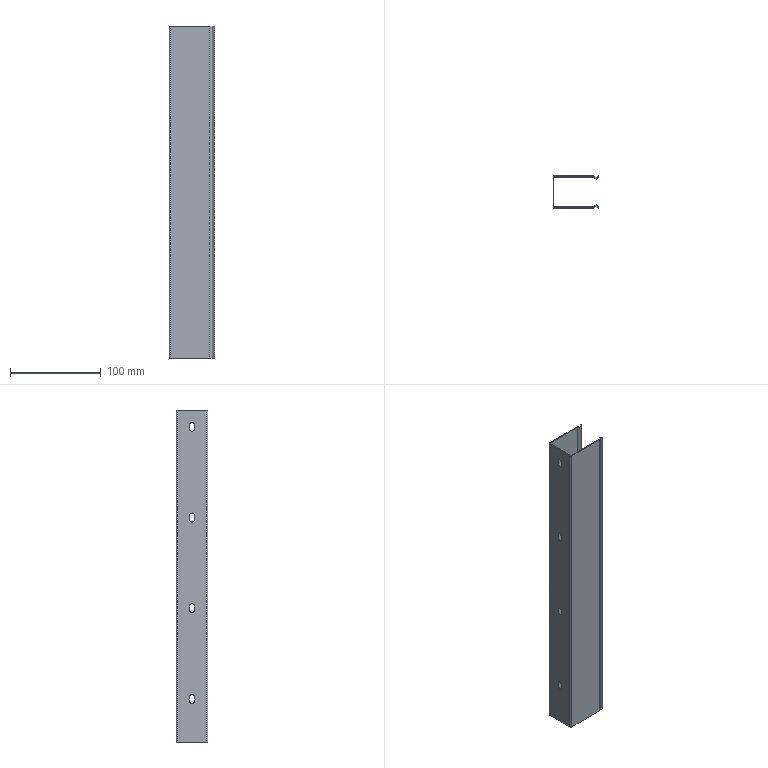Part | STEP file | 35 wire duct | 1 solid | 42 faces | box 50.625 x 35 x 366 mm | volume 49541 mm3 | plane 26 | cylinder 16 | commonest cylinder face diameters 5 x12 1 x2 3 x2